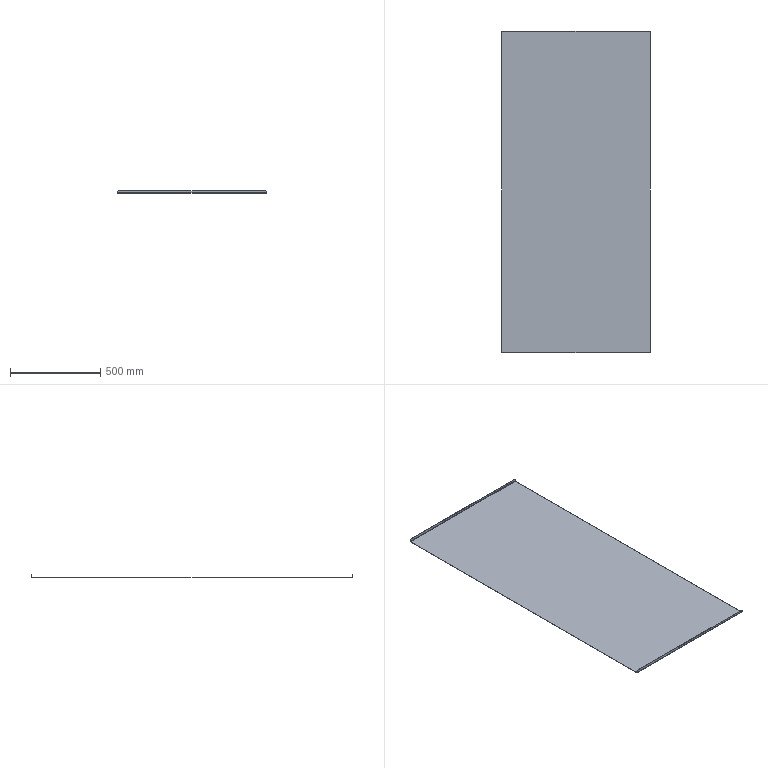Part | SolidWorks | features BaseBody 1 | 1 solid | 26 faces | box 819.9 x 1776 x 15 mm | volume 2215497 mm3 | plane 22 | cylinder 4 | commonest cylinder face diameters 2 x2 5 x2
STEP:
#1=CARTESIAN_POINT('',(-404.95,-888.,13.5));
#2=VERTEX_POINT('',#1);
#3=CARTESIAN_POINT('',(-409.95,-888.,8.5));
#4=VERTEX_POINT('',#3);
#5=CARTESIAN_POINT('',(-409.95,-888.,8.5));
#6=DIRECTION('',(-0.7071,0.,-0.7071));
#7=VECTOR('',#6,1000.);
#8=LINE('',#5,#7);
#9=EDGE_CURVE('',#2,#4,#8,.T.);
#10=ORIENTED_EDGE('',*,*,#9,.F.);
#11=CARTESIAN_POINT('',(-404.95,-886.5,13.5));
#12=VERTEX_POINT('',#11);
#13=CARTESIAN_POINT('',(-404.95,-888.,13.5));
#14=DIRECTION('',(0.,-1.,0.));
#15=VECTOR('',#14,1000.);
#16=LINE('',#13,#15);
#17=EDGE_CURVE('',#12,#2,#16,.T.);
#18=ORIENTED_EDGE('',*,*,#17,.F.);
#19=CARTESIAN_POINT('',(-409.95,-886.5,8.5));
#20=VERTEX_POINT('',#19);
#21=CARTESIAN_POINT('',(-209.225,-886.5,209.225));
#22=DIRECTION('',(0.7071,0.,0.7071));
#23=VECTOR('',#22,1000.);
#24=LINE('',#21,#23);
#25=EDGE_CURVE('',#20,#12,#24,.T.);
#26=ORIENTED_EDGE('',*,*,#25,.F.);
#27=CARTESIAN_POINT('',(-409.95,-888.,8.5));
#28=DIRECTION('',(0.,1.,0.));
#29=VECTOR('',#28,1000.);
#30=LINE('',#27,#29);
#31=EDGE_CURVE('',#4,#20,#30,.T.);
#32=ORIENTED_EDGE('',*,*,#31,.F.);
#33=EDGE_LOOP('',(#10,#18,#26,#32));
#34=FACE_OUTER_BOUND('',#33,.T.);
#35=CARTESIAN_POINT('',(-409.95,-888.,8.5));
#36=DIRECTION('',(0.7071,0.,-0.7071));
#37=DIRECTION('',(0.,-1.,0.));
#38=AXIS2_PLACEMENT_3D('',#35,#36,#37);
#39=PLANE('',#38);
#40=ADVANCED_FACE('',(#34),#39,.F.);
#41=CARTESIAN_POINT('',(409.95,-888.,8.5));
#42=VERTEX_POINT('',#41);
#43=CARTESIAN_POINT('',(404.95,-888.,13.5));
#44=VERTEX_POINT('',#43);
#45=CARTESIAN_POINT('',(404.95,-888.,13.5));
#46=DIRECTION('',(-0.7071,0.,0.7071));
#47=VECTOR('',#46,1000.);
#48=LINE('',#45,#47);
#49=EDGE_CURVE('',#42,#44,#48,.T.);
#50=ORIENTED_EDGE('',*,*,#49,.F.);
#51=CARTESIAN_POINT('',(409.95,-886.5,8.5));
#52=VERTEX_POINT('',#51);
#53=CARTESIAN_POINT('',(409.95,-888.,8.5));
#54=DIRECTION('',(0.,-1.,0.));
#55=VECTOR('',#54,1000.);
#56=LINE('',#53,#55);
#57=EDGE_CURVE('',#52,#42,#56,.T.);
#58=ORIENTED_EDGE('',*,*,#57,.F.);
#59=CARTESIAN_POINT('',(404.95,-886.5,13.5));
#60=VERTEX_POINT('',#59);
#61=CARTESIAN_POINT('',(209.225,-886.5,209.225));
#62=DIRECTION('',(0.7071,0.,-0.7071));
#63=VECTOR('',#62,1000.);
#64=LINE('',#61,#63);
#65=EDGE_CURVE('',#60,#52,#64,.T.);
#66=ORIENTED_EDGE('',*,*,#65,.F.);
#67=CARTESIAN_POINT('',(404.95,-888.,13.5));
#68=DIRECTION('',(0.,1.,0.));
#69=VECTOR('',#68,1000.);
#70=LINE('',#67,#69);
#71=EDGE_CURVE('',#44,#60,#70,.T.);
#72=ORIENTED_EDGE('',*,*,#71,.F.);
#73=EDGE_LOOP('',(#50,#58,#66,#72));
#74=FACE_OUTER_BOUND('',#73,.T.);
#75=CARTESIAN_POINT('',(404.95,-888.,13.5));
#76=DIRECTION('',(-0.7071,0.,-0.7071));
#77=DIRECTION('',(-0.7071,0.,0.7071));
#78=AXIS2_PLACEMENT_3D('',#75,#76,#77);
#79=PLANE('',#78);
#80=ADVANCED_FACE('',(#74),#79,.F.);
#81=CARTESIAN_POINT('',(404.95,888.,13.5));
#82=VERTEX_POINT('',#81);
#83=CARTESIAN_POINT('',(409.95,888.,8.5));
#84=VERTEX_POINT('',#83);
#85=CARTESIAN_POINT('',(409.95,888.,8.5));
#86=DIRECTION('',(0.7071,0.,-0.7071));
#87=VECTOR('',#86,1000.);
#88=LINE('',#85,#87);
#89=EDGE_CURVE('',#82,#84,#88,.T.);
#90=ORIENTED_EDGE('',*,*,#89,.F.);
#91=CARTESIAN_POINT('',(404.95,886.5,13.5));
#92=VERTEX_POINT('',#91);
#93=CARTESIAN_POINT('',(404.95,888.,13.5));
#94=DIRECTION('',(0.,1.,0.));
#95=VECTOR('',#94,1000.);
#96=LINE('',#93,#95);
#97=EDGE_CURVE('',#92,#82,#96,.T.);
#98=ORIENTED_EDGE('',*,*,#97,.F.);
#99=CARTESIAN_POINT('',(409.95,886.5,8.5));
#100=VERTEX_POINT('',#99);
#101=CARTESIAN_POINT('',(209.225,886.5,209.225));
#102=DIRECTION('',(-0.7071,0.,0.7071));
#103=VECTOR('',#102,1000.);
#104=LINE('',#101,#103);
#105=EDGE_CURVE('',#100,#92,#104,.T.);
#106=ORIENTED_EDGE('',*,*,#105,.F.);
#107=CARTESIAN_POINT('',(409.95,888.,8.5));
#108=DIRECTION('',(0.,-1.,0.));
#109=VECTOR('',#108,1000.);
#110=LINE('',#107,#109);
#111=EDGE_CURVE('',#84,#100,#110,.T.);
#112=ORIENTED_EDGE('',*,*,#111,.F.);
#113=EDGE_LOOP('',(#90,#98,#106,#112));
#114=FACE_OUTER_BOUND('',#113,.T.);
#115=CARTESIAN_POINT('',(409.95,888.,8.5));
#116=DIRECTION('',(-0.7071,0.,-0.7071));
#117=DIRECTION('',(-0.7071,0.,0.7071));
#118=AXIS2_PLACEMENT_3D('',#115,#116,#117);
#119=PLANE('',#118);
#120=ADVANCED_FACE('',(#114),#119,.F.);
#121=CARTESIAN_POINT('',(-409.95,888.,8.5));
#122=VERTEX_POINT('',#121);
#123=CARTESIAN_POINT('',(-404.95,888.,13.5));
#124=VERTEX_POINT('',#123);
#125=CARTESIAN_POINT('',(-404.95,888.,13.5));
#126=DIRECTION('',(0.7071,0.,0.7071));
#127=VECTOR('',#126,1000.);
#128=LINE('',#125,#127);
#129=EDGE_CURVE('',#122,#124,#128,.T.);
#130=ORIENTED_EDGE('',*,*,#129,.F.);
#131=CARTESIAN_POINT('',(-409.95,886.5,8.5));
#132=VERTEX_POINT('',#131);
#133=CARTESIAN_POINT('',(-409.95,888.,8.5));
#134=DIRECTION('',(0.,1.,0.));
#135=VECTOR('',#134,1000.);
#136=LINE('',#133,#135);
#137=EDGE_CURVE('',#132,#122,#136,.T.);
#138=ORIENTED_EDGE('',*,*,#137,.F.);
#139=CARTESIAN_POINT('',(-404.95,886.5,13.5));
#140=VERTEX_POINT('',#139);
#141=CARTESIAN_POINT('',(-209.225,886.5,209.225));
#142=DIRECTION('',(-0.7071,0.,-0.7071));
#143=VECTOR('',#142,1000.);
#144=LINE('',#141,#143);
#145=EDGE_CURVE('',#140,#132,#144,.T.);
#146=ORIENTED_EDGE('',*,*,#145,.F.);
#147=CARTESIAN_POINT('',(-404.95,888.,13.5));
#148=DIRECTION('',(0.,-1.,0.));
#149=VECTOR('',#148,1000.);
#150=LINE('',#147,#149);
#151=EDGE_CURVE('',#124,#140,#150,.T.);
#152=ORIENTED_EDGE('',*,*,#151,.F.);
#153=EDGE_LOOP('',(#130,#138,#146,#152));
#154=FACE_OUTER_BOUND('',#153,.T.);
#155=CARTESIAN_POINT('',(-404.95,888.,13.5));
#156=DIRECTION('',(0.7071,0.,-0.7071));
#157=DIRECTION('',(0.,-1.,0.));
#158=AXIS2_PLACEMENT_3D('',#155,#156,#157);
#159=PLANE('',#158);
#160=ADVANCED_FACE('',(#154),#159,.F.);
#161=CARTESIAN_POINT('',(0.,-888.,13.5));
#162=DIRECTION('',(-1.,0.,0.));
#163=VECTOR('',#162,1000.);
#164=LINE('',#161,#163);
#165=EDGE_CURVE('',#44,#2,#164,.T.);
#166=ORIENTED_EDGE('',*,*,#165,.F.);
#167=ORIENTED_EDGE('',*,*,#71,.T.);
#168=CARTESIAN_POINT('',(-409.95,-886.5,13.5));
#169=DIRECTION('',(-1.,0.,0.));
#170=VECTOR('',#169,1000.);
#171=LINE('',#168,#170);
#172=EDGE_CURVE('',#60,#12,#171,.T.);
#173=ORIENTED_EDGE('',*,*,#172,.T.);
#174=ORIENTED_EDGE('',*,*,#17,.T.);
#175=EDGE_LOOP('',(#166,#167,#173,#174));
#176=FACE_OUTER_BOUND('',#175,.T.);
#177=CARTESIAN_POINT('',(-409.95,-888.,13.5));
#178=DIRECTION('',(0.,0.,-1.));
#179=DIRECTION('',(-1.,0.,0.));
#180=AXIS2_PLACEMENT_3D('',#177,#178,#179);
#181=PLANE('',#180);
#182=ADVANCED_FACE('',(#176),#181,.F.);
#183=ORIENTED_EDGE('',*,*,#172,.F.);
#184=ORIENTED_EDGE('',*,*,#65,.T.);
#185=CARTESIAN_POINT('',(409.95,-886.5,1.));
#186=VERTEX_POINT('',#185);
#187=CARTESIAN_POINT('',(409.95,-886.5,13.5));
#188=DIRECTION('',(0.,0.,1.));
#189=VECTOR('',#188,1000.);
#190=LINE('',#187,#189);
#191=EDGE_CURVE('',#186,#52,#190,.T.);
#192=ORIENTED_EDGE('',*,*,#191,.F.);
#193=CARTESIAN_POINT('',(-409.95,-886.5,1.));
#194=VERTEX_POINT('',#193);
#195=CARTESIAN_POINT('',(-409.95,-886.5,1.));
#196=DIRECTION('',(1.,0.,0.));
#197=VECTOR('',#196,1000.);
#198=LINE('',#195,#197);
#199=EDGE_CURVE('',#194,#186,#198,.T.);
#200=ORIENTED_EDGE('',*,*,#199,.F.);
#201=CARTESIAN_POINT('',(-409.95,-886.5,0.));
#202=DIRECTION('',(0.,0.,-1.));
#203=VECTOR('',#202,1000.);
#204=LINE('',#201,#203);
#205=EDGE_CURVE('',#20,#194,#204,.T.);
#206=ORIENTED_EDGE('',*,*,#205,.F.);
#207=ORIENTED_EDGE('',*,*,#25,.T.);
#208=EDGE_LOOP('',(#183,#184,#192,#200,#206,#207));
#209=FACE_OUTER_BOUND('',#208,.T.);
#210=CARTESIAN_POINT('',(0.,-886.5,0.));
#211=DIRECTION('',(0.,1.,0.));
#212=DIRECTION('',(1.,0.,0.));
#213=AXIS2_PLACEMENT_3D('',#210,#211,#212);
#214=PLANE('',#213);
#215=ADVANCED_FACE('',(#209),#214,.T.);
#216=CARTESIAN_POINT('',(409.95,-888.,1.));
#217=VERTEX_POINT('',#216);
#218=CARTESIAN_POINT('',(409.95,-888.,0.));
#219=DIRECTION('',(0.,0.,1.));
#220=VECTOR('',#219,1000.);
#221=LINE('',#218,#220);
#222=EDGE_CURVE('',#217,#42,#221,.T.);
#223=ORIENTED_EDGE('',*,*,#222,.T.);
#224=ORIENTED_EDGE('',*,*,#49,.T.);
#225=ORIENTED_EDGE('',*,*,#165,.T.);
#226=ORIENTED_EDGE('',*,*,#9,.T.);
#227=CARTESIAN_POINT('',(-409.95,-888.,1.));
#228=VERTEX_POINT('',#227);
#229=CARTESIAN_POINT('',(-409.95,-888.,0.));
#230=DIRECTION('',(0.,0.,-1.));
#231=VECTOR('',#230,1000.);
#232=LINE('',#229,#231);
#233=EDGE_CURVE('',#4,#228,#232,.T.);
#234=ORIENTED_EDGE('',*,*,#233,.T.);
#235=CARTESIAN_POINT('',(-409.95,-888.,1.));
#236=DIRECTION('',(-1.,0.,0.));
#237=VECTOR('',#236,1000.);
#238=LINE('',#235,#237);
#239=EDGE_CURVE('',#217,#228,#238,.T.);
#240=ORIENTED_EDGE('',*,*,#239,.F.);
#241=EDGE_LOOP('',(#223,#224,#225,#226,#234,#240));
#242=FACE_OUTER_BOUND('',#241,.T.);
#243=CARTESIAN_POINT('',(0.,-888.,0.));
#244=DIRECTION('',(0.,1.,0.));
#245=DIRECTION('',(1.,0.,0.));
#246=AXIS2_PLACEMENT_3D('',#243,#244,#245);
#247=PLANE('',#246);
#248=ADVANCED_FACE('',(#242),#247,.F.);
#249=ORIENTED_EDGE('',*,*,#191,.T.);
#250=ORIENTED_EDGE('',*,*,#57,.T.);
#251=ORIENTED_EDGE('',*,*,#222,.F.);
#252=CARTESIAN_POINT('',(409.95,-886.5,1.));
#253=DIRECTION('',(0.,-1.,0.));
#254=VECTOR('',#253,1000.);
#255=LINE('',#252,#254);
#256=EDGE_CURVE('',#186,#217,#255,.T.);
#257=ORIENTED_EDGE('',*,*,#256,.F.);
#258=EDGE_LOOP('',(#249,#250,#251,#257));
#259=FACE_OUTER_BOUND('',#258,.T.);
#260=CARTESIAN_POINT('',(409.95,-888.,13.5));
#261=DIRECTION('',(-1.,0.,0.));
#262=DIRECTION('',(0.,0.,1.));
#263=AXIS2_PLACEMENT_3D('',#260,#261,#262);
#264=PLANE('',#263);
#265=ADVANCED_FACE('',(#259),#264,.F.);
#266=ORIENTED_EDGE('',*,*,#233,.F.);
#267=ORIENTED_EDGE('',*,*,#31,.T.);
#268=ORIENTED_EDGE('',*,*,#205,.T.);
#269=CARTESIAN_POINT('',(-409.95,-888.,1.));
#270=DIRECTION('',(0.,-1.,0.));
#271=VECTOR('',#270,1000.);
#272=LINE('',#269,#271);
#273=EDGE_CURVE('',#194,#228,#272,.T.);
#274=ORIENTED_EDGE('',*,*,#273,.T.);
#275=EDGE_LOOP('',(#266,#267,#268,#274));
#276=FACE_OUTER_BOUND('',#275,.T.);
#277=CARTESIAN_POINT('',(-409.95,-888.,0.));
#278=DIRECTION('',(1.,0.,0.));
#279=DIRECTION('',(0.,1.,0.));
#280=AXIS2_PLACEMENT_3D('',#277,#278,#279);
#281=PLANE('',#280);
#282=ADVANCED_FACE('',(#276),#281,.F.);
#283=CARTESIAN_POINT('',(409.95,-885.5,0.));
#284=VERTEX_POINT('',#283);
#285=CARTESIAN_POINT('',(-409.95,-885.5,0.));
#286=VERTEX_POINT('',#285);
#287=CARTESIAN_POINT('',(409.95,-885.5,0.));
#288=DIRECTION('',(-1.,0.,0.));
#289=VECTOR('',#288,1000.);
#290=LINE('',#287,#289);
#291=EDGE_CURVE('',#284,#286,#290,.T.);
#292=ORIENTED_EDGE('',*,*,#291,.T.);
#293=CARTESIAN_POINT('',(-409.95,-885.5,1.));
#294=DIRECTION('',(-1.,0.,0.));
#295=DIRECTION('',(0.,0.,-1.));
#296=AXIS2_PLACEMENT_3D('',#293,#294,#295);
#297=CIRCLE('',#296,1.);
#298=EDGE_CURVE('',#286,#194,#297,.T.);
#299=ORIENTED_EDGE('',*,*,#298,.T.);
#300=ORIENTED_EDGE('',*,*,#199,.T.);
#301=CARTESIAN_POINT('',(409.95,-885.5,1.));
#302=DIRECTION('',(1.,0.,0.));
#303=DIRECTION('',(0.,0.,-1.));
#304=AXIS2_PLACEMENT_3D('',#301,#302,#303);
#305=CIRCLE('',#304,1.);
#306=EDGE_CURVE('',#186,#284,#305,.T.);
#307=ORIENTED_EDGE('',*,*,#306,.T.);
#308=EDGE_LOOP('',(#292,#299,#300,#307));
#309=FACE_OUTER_BOUND('',#308,.T.);
#310=CARTESIAN_POINT('',(409.95,-885.5,1.));
#311=DIRECTION('',(1.,0.,0.));
#312=DIRECTION('',(0.,-1.,0.));
#313=AXIS2_PLACEMENT_3D('',#310,#311,#312);
#314=CYLINDRICAL_SURFACE('',#313,1.);
#315=ADVANCED_FACE('',(#309),#314,.F.);
#316=CARTESIAN_POINT('',(409.95,-885.5,-1.5));
#317=VERTEX_POINT('',#316);
#318=CARTESIAN_POINT('',(-409.95,-885.5,-1.5));
#319=VERTEX_POINT('',#318);
#320=CARTESIAN_POINT('',(409.95,-885.5,-1.5));
#321=DIRECTION('',(-1.,0.,0.));
#322=VECTOR('',#321,1000.);
#323=LINE('',#320,#322);
#324=EDGE_CURVE('',#317,#319,#323,.T.);
#325=ORIENTED_EDGE('',*,*,#324,.F.);
#326=CARTESIAN_POINT('',(409.95,-885.5,1.));
#327=DIRECTION('',(1.,0.,0.));
#328=DIRECTION('',(0.,0.,-1.));
#329=AXIS2_PLACEMENT_3D('',#326,#327,#328);
#330=CIRCLE('',#329,2.5);
#331=EDGE_CURVE('',#217,#317,#330,.T.);
#332=ORIENTED_EDGE('',*,*,#331,.F.);
#333=ORIENTED_EDGE('',*,*,#239,.T.);
#334=CARTESIAN_POINT('',(-409.95,-885.5,1.));
#335=DIRECTION('',(-1.,0.,0.));
#336=DIRECTION('',(0.,0.,-1.));
#337=AXIS2_PLACEMENT_3D('',#334,#335,#336);
#338=CIRCLE('',#337,2.5);
#339=EDGE_CURVE('',#319,#228,#338,.T.);
#340=ORIENTED_EDGE('',*,*,#339,.F.);
#341=EDGE_LOOP('',(#325,#332,#333,#340));
#342=FACE_OUTER_BOUND('',#341,.T.);
#343=CARTESIAN_POINT('',(409.95,-885.5,1.));
#344=DIRECTION('',(1.,0.,0.));
#345=DIRECTION('',(0.,-1.,0.));
#346=AXIS2_PLACEMENT_3D('',#343,#344,#345);
#347=CYLINDRICAL_SURFACE('',#346,2.5);
#348=ADVANCED_FACE('',(#342),#347,.T.);
#349=ORIENTED_EDGE('',*,*,#306,.F.);
#350=ORIENTED_EDGE('',*,*,#256,.T.);
#351=ORIENTED_EDGE('',*,*,#331,.T.);
#352=CARTESIAN_POINT('',(409.95,-885.5,0.));
#353=DIRECTION('',(0.,0.,-1.));
#354=VECTOR('',#353,1000.);
#355=LINE('',#352,#354);
#356=EDGE_CURVE('',#284,#317,#355,.T.);
#357=ORIENTED_EDGE('',*,*,#356,.F.);
#358=EDGE_LOOP('',(#349,#350,#351,#357));
#359=FACE_OUTER_BOUND('',#358,.T.);
#360=CARTESIAN_POINT('',(409.95,-885.5,1.));
#361=DIRECTION('',(-1.,0.,0.));
#362=DIRECTION('',(0.,0.,1.));
#363=AXIS2_PLACEMENT_3D('',#360,#361,#362);
#364=PLANE('',#363);
#365=ADVANCED_FACE('',(#359),#364,.F.);
#366=ORIENTED_EDGE('',*,*,#273,.F.);
#367=ORIENTED_EDGE('',*,*,#298,.F.);
#368=CARTESIAN_POINT('',(-409.95,-885.5,0.));
#369=DIRECTION('',(0.,0.,-1.));
#370=VECTOR('',#369,1000.);
#371=LINE('',#368,#370);
#372=EDGE_CURVE('',#286,#319,#371,.T.);
#373=ORIENTED_EDGE('',*,*,#372,.T.);
#374=ORIENTED_EDGE('',*,*,#339,.T.);
#375=EDGE_LOOP('',(#366,#367,#373,#374));
#376=FACE_OUTER_BOUND('',#375,.T.);
#377=CARTESIAN_POINT('',(-409.95,-885.5,1.));
#378=DIRECTION('',(-1.,0.,0.));
#379=DIRECTION('',(0.,0.,1.));
#380=AXIS2_PLACEMENT_3D('',#377,#378,#379);
#381=PLANE('',#380);
#382=ADVANCED_FACE('',(#376),#381,.T.);
#383=CARTESIAN_POINT('',(0.,888.,13.5));
#384=DIRECTION('',(1.,0.,0.));
#385=VECTOR('',#384,1000.);
#386=LINE('',#383,#385);
#387=EDGE_CURVE('',#124,#82,#386,.T.);
#388=ORIENTED_EDGE('',*,*,#387,.F.);
#389=ORIENTED_EDGE('',*,*,#151,.T.);
#390=CARTESIAN_POINT('',(409.95,886.5,13.5));
#391=DIRECTION('',(1.,0.,0.));
#392=VECTOR('',#391,1000.);
#393=LINE('',#390,#392);
#394=EDGE_CURVE('',#140,#92,#393,.T.);
#395=ORIENTED_EDGE('',*,*,#394,.T.);
#396=ORIENTED_EDGE('',*,*,#97,.T.);
#397=EDGE_LOOP('',(#388,#389,#395,#396));
#398=FACE_OUTER_BOUND('',#397,.T.);
#399=CARTESIAN_POINT('',(409.95,888.,13.5));
#400=DIRECTION('',(0.,0.,-1.));
#401=DIRECTION('',(0.,-1.,0.));
#402=AXIS2_PLACEMENT_3D('',#399,#400,#401);
#403=PLANE('',#402);
#404=ADVANCED_FACE('',(#398),#403,.F.);
#405=ORIENTED_EDGE('',*,*,#394,.F.);
#406=ORIENTED_EDGE('',*,*,#145,.T.);
#407=CARTESIAN_POINT('',(-409.95,886.5,1.));
#408=VERTEX_POINT('',#407);
#409=CARTESIAN_POINT('',(-409.95,886.5,13.5));
#410=DIRECTION('',(0.,0.,1.));
#411=VECTOR('',#410,1000.);
#412=LINE('',#409,#411);
#413=EDGE_CURVE('',#408,#132,#412,.T.);
#414=ORIENTED_EDGE('',*,*,#413,.F.);
#415=CARTESIAN_POINT('',(409.95,886.5,1.));
#416=VERTEX_POINT('',#415);
#417=CARTESIAN_POINT('',(409.95,886.5,1.));
#418=DIRECTION('',(-1.,0.,0.));
#419=VECTOR('',#418,1000.);
#420=LINE('',#417,#419);
#421=EDGE_CURVE('',#416,#408,#420,.T.);
#422=ORIENTED_EDGE('',*,*,#421,.F.);
#423=CARTESIAN_POINT('',(409.95,886.5,0.));
#424=DIRECTION('',(0.,0.,-1.));
#425=VECTOR('',#424,1000.);
#426=LINE('',#423,#425);
#427=EDGE_CURVE('',#100,#416,#426,.T.);
#428=ORIENTED_EDGE('',*,*,#427,.F.);
#429=ORIENTED_EDGE('',*,*,#105,.T.);
#430=EDGE_LOOP('',(#405,#406,#414,#422,#428,#429));
#431=FACE_OUTER_BOUND('',#430,.T.);
#432=CARTESIAN_POINT('',(0.,886.5,0.));
#433=DIRECTION('',(0.,-1.,0.));
#434=DIRECTION('',(-1.,0.,0.));
#435=AXIS2_PLACEMENT_3D('',#432,#433,#434);
#436=PLANE('',#435);
#437=ADVANCED_FACE('',(#431),#436,.T.);
#438=CARTESIAN_POINT('',(-409.95,888.,1.));
#439=VERTEX_POINT('',#438);
#440=CARTESIAN_POINT('',(-409.95,888.,0.));
#441=DIRECTION('',(0.,0.,1.));
#442=VECTOR('',#441,1000.);
#443=LINE('',#440,#442);
#444=EDGE_CURVE('',#439,#122,#443,.T.);
#445=ORIENTED_EDGE('',*,*,#444,.T.);
#446=ORIENTED_EDGE('',*,*,#129,.T.);
#447=ORIENTED_EDGE('',*,*,#387,.T.);
#448=ORIENTED_EDGE('',*,*,#89,.T.);
#449=CARTESIAN_POINT('',(409.95,888.,1.));
#450=VERTEX_POINT('',#449);
#451=CARTESIAN_POINT('',(409.95,888.,0.));
#452=DIRECTION('',(0.,0.,-1.));
#453=VECTOR('',#452,1000.);
#454=LINE('',#451,#453);
#455=EDGE_CURVE('',#84,#450,#454,.T.);
#456=ORIENTED_EDGE('',*,*,#455,.T.);
#457=CARTESIAN_POINT('',(409.95,888.,1.));
#458=DIRECTION('',(1.,0.,0.));
#459=VECTOR('',#458,1000.);
#460=LINE('',#457,#459);
#461=EDGE_CURVE('',#439,#450,#460,.T.);
#462=ORIENTED_EDGE('',*,*,#461,.F.);
#463=EDGE_LOOP('',(#445,#446,#447,#448,#456,#462));
#464=FACE_OUTER_BOUND('',#463,.T.);
#465=CARTESIAN_POINT('',(0.,888.,0.));
#466=DIRECTION('',(0.,-1.,0.));
#467=DIRECTION('',(-1.,0.,0.));
#468=AXIS2_PLACEMENT_3D('',#465,#466,#467);
#469=PLANE('',#468);
#470=ADVANCED_FACE('',(#464),#469,.F.);
#471=ORIENTED_EDGE('',*,*,#413,.T.);
#472=ORIENTED_EDGE('',*,*,#137,.T.);
#473=ORIENTED_EDGE('',*,*,#444,.F.);
#474=CARTESIAN_POINT('',(-409.95,886.5,1.));
#475=DIRECTION('',(0.,1.,0.));
#476=VECTOR('',#475,1000.);
#477=LINE('',#474,#476);
#478=EDGE_CURVE('',#408,#439,#477,.T.);
#479=ORIENTED_EDGE('',*,*,#478,.F.);
#480=EDGE_LOOP('',(#471,#472,#473,#479));
#481=FACE_OUTER_BOUND('',#480,.T.);
#482=CARTESIAN_POINT('',(-409.95,888.,13.5));
#483=DIRECTION('',(1.,0.,0.));
#484=DIRECTION('',(0.,1.,0.));
#485=AXIS2_PLACEMENT_3D('',#482,#483,#484);
#486=PLANE('',#485);
#487=ADVANCED_FACE('',(#481),#486,.F.);
#488=ORIENTED_EDGE('',*,*,#455,.F.);
#489=ORIENTED_EDGE('',*,*,#111,.T.);
#490=ORIENTED_EDGE('',*,*,#427,.T.);
#491=CARTESIAN_POINT('',(409.95,888.,1.));
#492=DIRECTION('',(0.,1.,0.));
#493=VECTOR('',#492,1000.);
#494=LINE('',#491,#493);
#495=EDGE_CURVE('',#416,#450,#494,.T.);
#496=ORIENTED_EDGE('',*,*,#495,.T.);
#497=EDGE_LOOP('',(#488,#489,#490,#496));
#498=FACE_OUTER_BOUND('',#497,.T.);
#499=CARTESIAN_POINT('',(409.95,888.,0.));
#500=DIRECTION('',(-1.,0.,0.));
#501=DIRECTION('',(0.,1.,0.));
#502=AXIS2_PLACEMENT_3D('',#499,#500,#501);
#503=PLANE('',#502);
#504=ADVANCED_FACE('',(#498),#503,.F.);
#505=CARTESIAN_POINT('',(-409.95,885.5,0.));
#506=VERTEX_POINT('',#505);
#507=CARTESIAN_POINT('',(409.95,885.5,0.));
#508=VERTEX_POINT('',#507);
#509=CARTESIAN_POINT('',(-409.95,885.5,0.));
#510=DIRECTION('',(1.,0.,0.));
#511=VECTOR('',#510,1000.);
#512=LINE('',#509,#511);
#513=EDGE_CURVE('',#506,#508,#512,.T.);
#514=ORIENTED_EDGE('',*,*,#513,.T.);
#515=CARTESIAN_POINT('',(409.95,885.5,1.));
#516=DIRECTION('',(1.,0.,0.));
#517=DIRECTION('',(0.,0.,1.));
#518=AXIS2_PLACEMENT_3D('',#515,#516,#517);
#519=CIRCLE('',#518,1.);
#520=EDGE_CURVE('',#508,#416,#519,.T.);
#521=ORIENTED_EDGE('',*,*,#520,.T.);
#522=ORIENTED_EDGE('',*,*,#421,.T.);
#523=CARTESIAN_POINT('',(-409.95,885.5,1.));
#524=DIRECTION('',(-1.,0.,0.));
#525=DIRECTION('',(0.,0.,1.));
#526=AXIS2_PLACEMENT_3D('',#523,#524,#525);
#527=CIRCLE('',#526,1.);
#528=EDGE_CURVE('',#408,#506,#527,.T.);
#529=ORIENTED_EDGE('',*,*,#528,.T.);
#530=EDGE_LOOP('',(#514,#521,#522,#529));
#531=FACE_OUTER_BOUND('',#530,.T.);
#532=CARTESIAN_POINT('',(-409.95,885.5,1.));
#533=DIRECTION('',(-1.,0.,0.));
#534=DIRECTION('',(0.,1.,0.));
#535=AXIS2_PLACEMENT_3D('',#532,#533,#534);
#536=CYLINDRICAL_SURFACE('',#535,1.);
#537=ADVANCED_FACE('',(#531),#536,.F.);
#538=CARTESIAN_POINT('',(-409.95,885.5,-1.5));
#539=VERTEX_POINT('',#538);
#540=CARTESIAN_POINT('',(409.95,885.5,-1.5));
#541=VERTEX_POINT('',#540);
#542=CARTESIAN_POINT('',(-409.95,885.5,-1.5));
#543=DIRECTION('',(1.,0.,0.));
#544=VECTOR('',#543,1000.);
#545=LINE('',#542,#544);
#546=EDGE_CURVE('',#539,#541,#545,.T.);
#547=ORIENTED_EDGE('',*,*,#546,.F.);
#548=CARTESIAN_POINT('',(-409.95,885.5,1.));
#549=DIRECTION('',(-1.,0.,0.));
#550=DIRECTION('',(0.,0.,1.));
#551=AXIS2_PLACEMENT_3D('',#548,#549,#550);
#552=CIRCLE('',#551,2.5);
#553=EDGE_CURVE('',#439,#539,#552,.T.);
#554=ORIENTED_EDGE('',*,*,#553,.F.);
#555=ORIENTED_EDGE('',*,*,#461,.T.);
#556=CARTESIAN_POINT('',(409.95,885.5,1.));
#557=DIRECTION('',(1.,0.,0.));
#558=DIRECTION('',(0.,0.,1.));
#559=AXIS2_PLACEMENT_3D('',#556,#557,#558);
#560=CIRCLE('',#559,2.5);
#561=EDGE_CURVE('',#541,#450,#560,.T.);
#562=ORIENTED_EDGE('',*,*,#561,.F.);
#563=EDGE_LOOP('',(#547,#554,#555,#562));
#564=FACE_OUTER_BOUND('',#563,.T.);
#565=CARTESIAN_POINT('',(-409.95,885.5,1.));
#566=DIRECTION('',(-1.,0.,0.));
#567=DIRECTION('',(0.,1.,0.));
#568=AXIS2_PLACEMENT_3D('',#565,#566,#567);
#569=CYLINDRICAL_SURFACE('',#568,2.5);
#570=ADVANCED_FACE('',(#564),#569,.T.);
#571=ORIENTED_EDGE('',*,*,#528,.F.);
#572=ORIENTED_EDGE('',*,*,#478,.T.);
#573=ORIENTED_EDGE('',*,*,#553,.T.);
#574=CARTESIAN_POINT('',(-409.95,885.5,0.));
#575=DIRECTION('',(0.,0.,-1.));
#576=VECTOR('',#575,1000.);
#577=LINE('',#574,#576);
#578=EDGE_CURVE('',#506,#539,#577,.T.);
#579=ORIENTED_EDGE('',*,*,#578,.F.);
#580=EDGE_LOOP('',(#571,#572,#573,#579));
#581=FACE_OUTER_BOUND('',#580,.T.);
#582=CARTESIAN_POINT('',(-409.95,885.5,1.));
#583=DIRECTION('',(1.,0.,0.));
#584=DIRECTION('',(0.,0.,1.));
#585=AXIS2_PLACEMENT_3D('',#582,#583,#584);
#586=PLANE('',#585);
#587=ADVANCED_FACE('',(#581),#586,.F.);
#588=ORIENTED_EDGE('',*,*,#495,.F.);
#589=ORIENTED_EDGE('',*,*,#520,.F.);
#590=CARTESIAN_POINT('',(409.95,885.5,0.));
#591=DIRECTION('',(0.,0.,-1.));
#592=VECTOR('',#591,1000.);
#593=LINE('',#590,#592);
#594=EDGE_CURVE('',#508,#541,#593,.T.);
#595=ORIENTED_EDGE('',*,*,#594,.T.);
#596=ORIENTED_EDGE('',*,*,#561,.T.);
#597=EDGE_LOOP('',(#588,#589,#595,#596));
#598=FACE_OUTER_BOUND('',#597,.T.);
#599=CARTESIAN_POINT('',(409.95,885.5,1.));
#600=DIRECTION('',(1.,0.,0.));
#601=DIRECTION('',(0.,0.,1.));
#602=AXIS2_PLACEMENT_3D('',#599,#600,#601);
#603=PLANE('',#602);
#604=ADVANCED_FACE('',(#598),#603,.T.);
#605=ORIENTED_EDGE('',*,*,#372,.F.);
#606=CARTESIAN_POINT('',(-409.95,888.,0.));
#607=DIRECTION('',(0.,-1.,0.));
#608=VECTOR('',#607,1000.);
#609=LINE('',#606,#608);
#610=EDGE_CURVE('',#506,#286,#609,.T.);
#611=ORIENTED_EDGE('',*,*,#610,.F.);
#612=ORIENTED_EDGE('',*,*,#578,.T.);
#613=CARTESIAN_POINT('',(-409.95,888.,-1.5));
#614=DIRECTION('',(0.,-1.,0.));
#615=VECTOR('',#614,1000.);
#616=LINE('',#613,#615);
#617=EDGE_CURVE('',#539,#319,#616,.T.);
#618=ORIENTED_EDGE('',*,*,#617,.T.);
#619=EDGE_LOOP('',(#605,#611,#612,#618));
#620=FACE_OUTER_BOUND('',#619,.T.);
#621=CARTESIAN_POINT('',(-409.95,888.,-1.5));
#622=DIRECTION('',(-1.,0.,0.));
#623=DIRECTION('',(0.,1.,0.));
#624=AXIS2_PLACEMENT_3D('',#621,#622,#623);
#625=PLANE('',#624);
#626=ADVANCED_FACE('',(#620),#625,.T.);
#627=CARTESIAN_POINT('',(409.95,888.,0.));
#628=DIRECTION('',(0.,1.,0.));
#629=VECTOR('',#628,1000.);
#630=LINE('',#627,#629);
#631=EDGE_CURVE('',#284,#508,#630,.T.);
#632=ORIENTED_EDGE('',*,*,#631,.F.);
#633=ORIENTED_EDGE('',*,*,#356,.T.);
#634=CARTESIAN_POINT('',(409.95,888.,-1.5));
#635=DIRECTION('',(0.,1.,0.));
#636=VECTOR('',#635,1000.);
#637=LINE('',#634,#636);
#638=EDGE_CURVE('',#317,#541,#637,.T.);
#639=ORIENTED_EDGE('',*,*,#638,.T.);
#640=ORIENTED_EDGE('',*,*,#594,.F.);
#641=EDGE_LOOP('',(#632,#633,#639,#640));
#642=FACE_OUTER_BOUND('',#641,.T.);
#643=CARTESIAN_POINT('',(409.95,888.,-1.5));
#644=DIRECTION('',(1.,0.,0.));
#645=DIRECTION('',(0.,1.,0.));
#646=AXIS2_PLACEMENT_3D('',#643,#644,#645);
#647=PLANE('',#646);
#648=ADVANCED_FACE('',(#642),#647,.T.);
#649=ORIENTED_EDGE('',*,*,#291,.F.);
#650=ORIENTED_EDGE('',*,*,#631,.T.);
#651=ORIENTED_EDGE('',*,*,#513,.F.);
#652=ORIENTED_EDGE('',*,*,#610,.T.);
#653=EDGE_LOOP('',(#649,#650,#651,#652));
#654=FACE_OUTER_BOUND('',#653,.T.);
#655=CARTESIAN_POINT('',(0.,0.,0.));
#656=DIRECTION('',(0.,0.,-1.));
#657=DIRECTION('',(0.,-1.,0.));
#658=AXIS2_PLACEMENT_3D('',#655,#656,#657);
#659=PLANE('',#658);
#660=ADVANCED_FACE('',(#654),#659,.F.);
#661=ORIENTED_EDGE('',*,*,#638,.F.);
#662=ORIENTED_EDGE('',*,*,#324,.T.);
#663=ORIENTED_EDGE('',*,*,#617,.F.);
#664=ORIENTED_EDGE('',*,*,#546,.T.);
#665=EDGE_LOOP('',(#661,#662,#663,#664));
#666=FACE_OUTER_BOUND('',#665,.T.);
#667=CARTESIAN_POINT('',(0.,0.,-1.5));
#668=DIRECTION('',(0.,0.,-1.));
#669=DIRECTION('',(0.,-1.,0.));
#670=AXIS2_PLACEMENT_3D('',#667,#668,#669);
#671=PLANE('',#670);
#672=ADVANCED_FACE('',(#666),#671,.T.);
#673=CLOSED_SHELL('',(#40,#80,#120,#160,#182,#215,#248,#265,#282,#315,#348,#365,#382,#404,#437,#470,#487,#504,#537,#570,#587,#604,#626,#648,#660,#672));
#674=MANIFOLD_SOLID_BREP('',#673);
#675=CARTESIAN_POINT('',(0.,0.,0.));
#676=DIRECTION('',(0.,0.,1.));
#677=DIRECTION('',(1.,0.,0.));
#678=AXIS2_PLACEMENT_3D('',#675,#676,#677);
#679=(LENGTH_UNIT()NAMED_UNIT(*)SI_UNIT(.MILLI.,.METRE.));
#680=UNCERTAINTY_MEASURE_WITH_UNIT(LENGTH_MEASURE(0.00001),#679,'','');
#681=(NAMED_UNIT(*)PLANE_ANGLE_UNIT()SI_UNIT($,.RADIAN.));
#682=(NAMED_UNIT(*)SI_UNIT($,.STERADIAN.)SOLID_ANGLE_UNIT());
#683=(GEOMETRIC_REPRESENTATION_CONTEXT(3)GLOBAL_UNCERTAINTY_ASSIGNED_CONTEXT((#680))GLOBAL_UNIT_ASSIGNED_CONTEXT((#679,#681,#682))REPRESENTATION_CONTEXT('',''));
#684=ADVANCED_BREP_SHAPE_REPRESENTATION('',(#674,#678),#683);